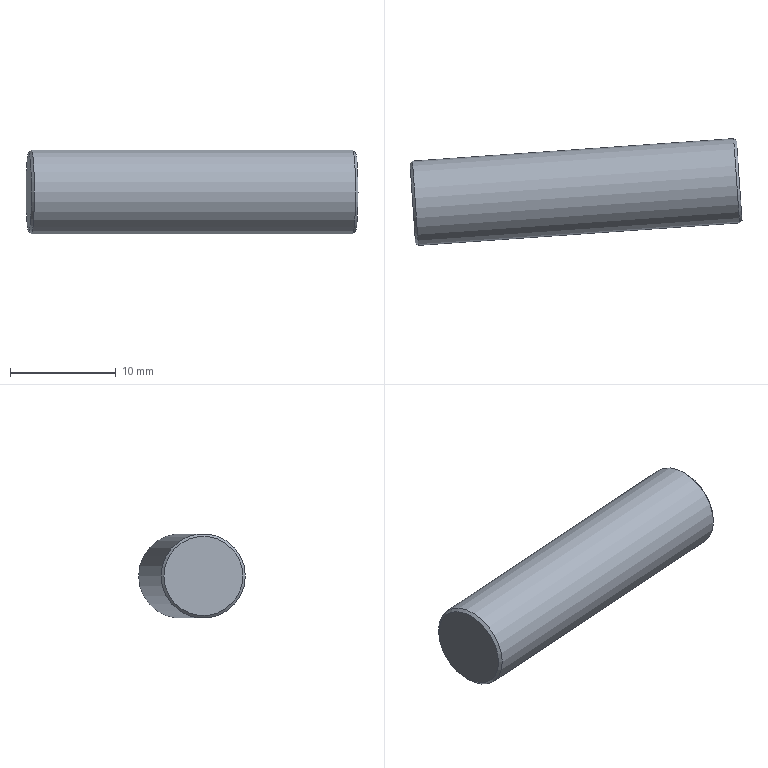Part | STEP file | 车灯-后视镜_id206_x_t | 1 solid | 5 faces | box 31.448 x 10.108 x 8 mm | volume 1557 mm3 | plane 2 | cone 2 | cylinder 1 | commonest cylinder face diameters 8 x1
STEP:
#1=CARTESIAN_POINT('',(18.033,-80.085,-237.501));
#2=VERTEX_POINT('',#1);
#3=CARTESIAN_POINT('',(18.295,-83.826,-237.501));
#4=DIRECTION('',(0.9976,0.06976,0.));
#5=DIRECTION('',(-0.06976,0.9976,0.));
#6=AXIS2_PLACEMENT_3D('',#3,#4,#5);
#7=CIRCLE('',#6,3.75);
#8=EDGE_CURVE('',#2,#2,#7,.T.);
#9=ORIENTED_EDGE('',*,*,#8,.T.);
#10=EDGE_LOOP('',(#9));
#11=FACE_OUTER_BOUND('',#10,.T.);
#12=CARTESIAN_POINT('',(18.235,-82.968,-255.5));
#13=DIRECTION('',(0.9976,0.06976,0.));
#14=DIRECTION('',(0.,0.,-1.));
#15=AXIS2_PLACEMENT_3D('',#12,#13,#14);
#16=PLANE('',#15);
#17=ADVANCED_FACE('',(#11),#16,.T.);
#18=CARTESIAN_POINT('',(17.766,-79.853,-237.501));
#19=VERTEX_POINT('',#18);
#20=CARTESIAN_POINT('',(18.045,-83.843,-237.501));
#21=DIRECTION('',(-0.9976,-0.06976,0.));
#22=DIRECTION('',(-0.06976,0.9976,0.));
#23=AXIS2_PLACEMENT_3D('',#20,#21,#22);
#24=CIRCLE('',#23,4.);
#25=EDGE_CURVE('',#19,#19,#24,.T.);
#26=ORIENTED_EDGE('',*,*,#25,.T.);
#27=EDGE_LOOP('',(#26));
#28=FACE_BOUND('',#27,.T.);
#29=CARTESIAN_POINT('',(-12.659,-81.981,-237.501));
#30=VERTEX_POINT('',#29);
#31=CARTESIAN_POINT('',(-12.38,-85.971,-237.501));
#32=DIRECTION('',(0.9976,0.06976,0.));
#33=DIRECTION('',(-0.06976,0.9976,0.));
#34=AXIS2_PLACEMENT_3D('',#31,#32,#33);
#35=CIRCLE('',#34,4.);
#36=EDGE_CURVE('',#30,#30,#35,.T.);
#37=ORIENTED_EDGE('',*,*,#36,.T.);
#38=EDGE_LOOP('',(#37));
#39=FACE_BOUND('',#38,.T.);
#40=CARTESIAN_POINT('',(-13.627,-86.058,-237.501));
#41=DIRECTION('',(0.9976,0.06976,0.));
#42=DIRECTION('',(-0.06976,0.9976,0.));
#43=AXIS2_PLACEMENT_3D('',#40,#41,#42);
#44=CYLINDRICAL_SURFACE('',#43,4.);
#45=ADVANCED_FACE('',(#28,#39),#44,.T.);
#46=CARTESIAN_POINT('',(-12.368,-89.729,-237.501));
#47=VERTEX_POINT('',#46);
#48=CARTESIAN_POINT('',(-12.63,-85.988,-237.501));
#49=DIRECTION('',(-0.9976,-0.06976,0.));
#50=DIRECTION('',(0.06976,-0.9976,0.));
#51=AXIS2_PLACEMENT_3D('',#48,#49,#50);
#52=CIRCLE('',#51,3.75);
#53=EDGE_CURVE('',#47,#47,#52,.T.);
#54=ORIENTED_EDGE('',*,*,#53,.T.);
#55=EDGE_LOOP('',(#54));
#56=FACE_OUTER_BOUND('',#55,.T.);
#57=CARTESIAN_POINT('',(-12.69,-85.13,-255.5));
#58=DIRECTION('',(-0.9976,-0.06976,0.));
#59=DIRECTION('',(0.,0.,1.));
#60=AXIS2_PLACEMENT_3D('',#57,#58,#59);
#61=PLANE('',#60);
#62=ADVANCED_FACE('',(#56),#61,.T.);
#63=ORIENTED_EDGE('',*,*,#25,.F.);
#64=EDGE_LOOP('',(#63));
#65=FACE_BOUND('',#64,.T.);
#66=ORIENTED_EDGE('',*,*,#8,.F.);
#67=EDGE_LOOP('',(#66));
#68=FACE_BOUND('',#67,.T.);
#69=CARTESIAN_POINT('',(18.295,-83.826,-237.501));
#70=DIRECTION('',(-0.9976,-0.06976,0.));
#71=DIRECTION('',(0.06976,-0.9976,0.));
#72=AXIS2_PLACEMENT_3D('',#69,#70,#71);
#73=CONICAL_SURFACE('',#72,3.75,45.);
#74=ADVANCED_FACE('',(#65,#68),#73,.T.);
#75=ORIENTED_EDGE('',*,*,#53,.F.);
#76=EDGE_LOOP('',(#75));
#77=FACE_BOUND('',#76,.T.);
#78=ORIENTED_EDGE('',*,*,#36,.F.);
#79=EDGE_LOOP('',(#78));
#80=FACE_BOUND('',#79,.T.);
#81=CARTESIAN_POINT('',(-12.38,-85.971,-237.501));
#82=DIRECTION('',(0.9976,0.06976,0.));
#83=DIRECTION('',(-0.06976,0.9976,0.));
#84=AXIS2_PLACEMENT_3D('',#81,#82,#83);
#85=CONICAL_SURFACE('',#84,4.,45.);
#86=ADVANCED_FACE('',(#77,#80),#85,.T.);
#87=CLOSED_SHELL('',(#17,#45,#62,#74,#86));
#88=MANIFOLD_SOLID_BREP('',#87);
#89=(LENGTH_UNIT()NAMED_UNIT(*)SI_UNIT(.MILLI.,.METRE.));
#90=UNCERTAINTY_MEASURE_WITH_UNIT(LENGTH_MEASURE(0.00002),#89,'','');
#91=(NAMED_UNIT(*)PLANE_ANGLE_UNIT()SI_UNIT($,.RADIAN.));
#92=PLANE_ANGLE_MEASURE_WITH_UNIT(PLANE_ANGLE_MEASURE(0.01745),#91);
#93=DIMENSIONAL_EXPONENTS(0.,0.,0.,0.,0.,0.,0.);
#94=(CONVERSION_BASED_UNIT('DEGREE',#92)NAMED_UNIT(#93)PLANE_ANGLE_UNIT());
#95=(NAMED_UNIT(*)SI_UNIT($,.STERADIAN.)SOLID_ANGLE_UNIT());
#96=(GEOMETRIC_REPRESENTATION_CONTEXT(3)GLOBAL_UNCERTAINTY_ASSIGNED_CONTEXT((#90))GLOBAL_UNIT_ASSIGNED_CONTEXT((#89,#94,#95))REPRESENTATION_CONTEXT('',''));
#97=ADVANCED_BREP_SHAPE_REPRESENTATION('',(#88),#96);